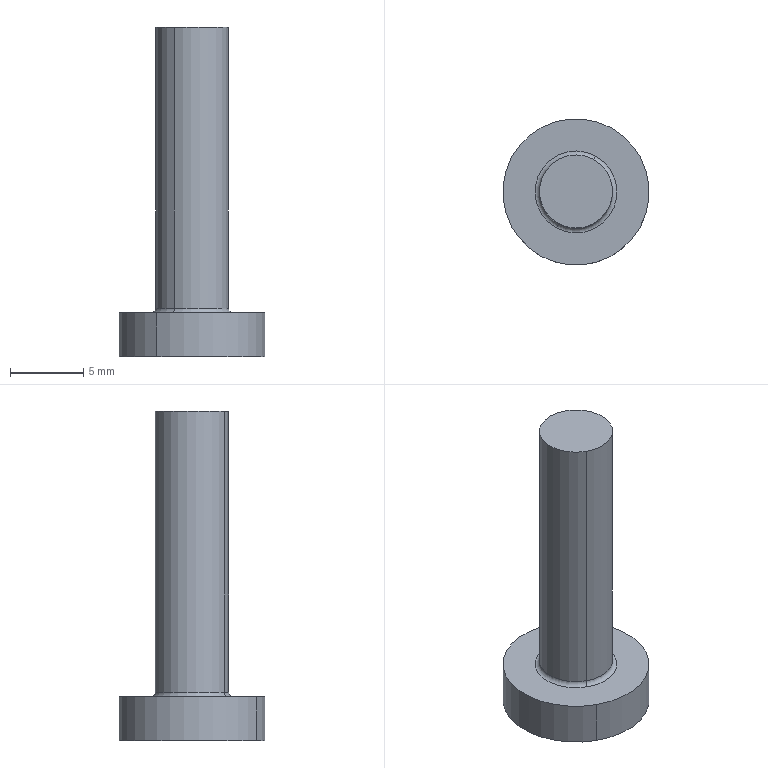Part | CATIA | 1 solid | 9 faces | box 10 x 10 x 22.5 mm | volume 618.813 mm3 | cylinder 4 | plane 3 | torus 2 | commonest cylinder face diameters 5 x2 10 x2
STEP:
#1=CARTESIAN_POINT('',(2.397,4.388,-3.));
#2=VERTEX_POINT('',#1);
#3=CARTESIAN_POINT('',(-2.397,-4.388,-3.));
#4=VERTEX_POINT('',#3);
#5=CARTESIAN_POINT('',(0.,0.,-3.));
#6=DIRECTION('',(0.,0.,-1.));
#7=AXIS2_PLACEMENT_3D('',#5,#6,$);
#8=CIRCLE('',#7,5.);
#9=EDGE_CURVE('',#2,#4,#8,.T.);
#10=ORIENTED_EDGE('',*,*,#9,.F.);
#11=CARTESIAN_POINT('',(2.397,4.388,0.));
#12=VERTEX_POINT('',#11);
#13=CARTESIAN_POINT('',(2.397,4.388,-1.5));
#14=DIRECTION('',(0.,0.,-1.));
#15=VECTOR('',#14,1.);
#16=LINE('',#13,#15);
#17=EDGE_CURVE('',#2,#12,#16,.F.);
#18=ORIENTED_EDGE('',*,*,#17,.T.);
#19=CARTESIAN_POINT('',(-2.397,-4.388,0.));
#20=VERTEX_POINT('',#19);
#21=CARTESIAN_POINT('',(0.,0.,0.));
#22=DIRECTION('',(0.,0.,-1.));
#23=AXIS2_PLACEMENT_3D('',#21,#22,$);
#24=CIRCLE('',#23,5.);
#25=EDGE_CURVE('',#12,#20,#24,.T.);
#26=ORIENTED_EDGE('',*,*,#25,.T.);
#27=CARTESIAN_POINT('',(-2.397,-4.388,-1.5));
#28=DIRECTION('',(0.,0.,-1.));
#29=VECTOR('',#28,1.);
#30=LINE('',#27,#29);
#31=EDGE_CURVE('',#4,#20,#30,.F.);
#32=ORIENTED_EDGE('',*,*,#31,.F.);
#33=EDGE_LOOP('',(#10,#18,#26,#32));
#34=FACE_OUTER_BOUND('',#33,.T.);
#35=CARTESIAN_POINT('',(0.,0.,8.25));
#36=DIRECTION('',(0.,0.,-1.));
#37=DIRECTION('',(0.4794,0.8776,0.));
#38=AXIS2_PLACEMENT_3D('',#35,#36,#37);
#39=CYLINDRICAL_SURFACE('',#38,5.);
#40=ADVANCED_FACE('',(#34),#39,.T.);
#41=CARTESIAN_POINT('',(0.,0.,-3.));
#42=DIRECTION('',(0.,0.,-1.));
#43=AXIS2_PLACEMENT_3D('',#41,#42,$);
#44=CIRCLE('',#43,5.);
#45=EDGE_CURVE('',#4,#2,#44,.T.);
#46=ORIENTED_EDGE('',*,*,#45,.F.);
#47=ORIENTED_EDGE('',*,*,#31,.T.);
#48=CARTESIAN_POINT('',(0.,0.,0.));
#49=DIRECTION('',(0.,0.,-1.));
#50=AXIS2_PLACEMENT_3D('',#48,#49,$);
#51=CIRCLE('',#50,5.);
#52=EDGE_CURVE('',#20,#12,#51,.T.);
#53=ORIENTED_EDGE('',*,*,#52,.T.);
#54=ORIENTED_EDGE('',*,*,#17,.F.);
#55=EDGE_LOOP('',(#46,#47,#53,#54));
#56=FACE_OUTER_BOUND('',#55,.T.);
#57=ADVANCED_FACE('',(#56),#39,.T.);
#58=CARTESIAN_POINT('',(1.342,2.457,0.));
#59=VERTEX_POINT('',#58);
#60=CARTESIAN_POINT('',(-1.342,-2.457,0.));
#61=VERTEX_POINT('',#60);
#62=CARTESIAN_POINT('',(0.,0.,0.));
#63=DIRECTION('',(0.,0.,-1.));
#64=AXIS2_PLACEMENT_3D('',#62,#63,$);
#65=CIRCLE('',#64,2.8);
#66=EDGE_CURVE('',#59,#61,#65,.T.);
#67=ORIENTED_EDGE('',*,*,#66,.F.);
#68=CARTESIAN_POINT('',(1.199,2.194,0.3));
#69=VERTEX_POINT('',#68);
#70=CARTESIAN_POINT('',(1.342,2.457,0.3));
#71=DIRECTION('',(-0.8776,0.4794,0.));
#72=AXIS2_PLACEMENT_3D('',#70,#71,$);
#73=CIRCLE('',#72,0.3);
#74=EDGE_CURVE('',#59,#69,#73,.T.);
#75=ORIENTED_EDGE('',*,*,#74,.T.);
#76=CARTESIAN_POINT('',(-1.199,-2.194,0.3));
#77=VERTEX_POINT('',#76);
#78=CARTESIAN_POINT('',(0.,0.,0.3));
#79=DIRECTION('',(0.,0.,-1.));
#80=AXIS2_PLACEMENT_3D('',#78,#79,$);
#81=CIRCLE('',#80,2.5);
#82=EDGE_CURVE('',#69,#77,#81,.T.);
#83=ORIENTED_EDGE('',*,*,#82,.T.);
#84=CARTESIAN_POINT('',(-1.342,-2.457,0.3));
#85=DIRECTION('',(0.8776,-0.4794,0.));
#86=AXIS2_PLACEMENT_3D('',#84,#85,$);
#87=CIRCLE('',#86,0.3);
#88=EDGE_CURVE('',#61,#77,#87,.T.);
#89=ORIENTED_EDGE('',*,*,#88,.F.);
#90=EDGE_LOOP('',(#67,#75,#83,#89));
#91=FACE_OUTER_BOUND('',#90,.T.);
#92=CARTESIAN_POINT('',(0.,0.,0.3));
#93=DIRECTION('',(0.,0.,-1.));
#94=DIRECTION('',(0.4794,0.8776,0.));
#95=AXIS2_PLACEMENT_3D('',#92,#93,#94);
#96=TOROIDAL_SURFACE('',#95,2.8,0.3);
#97=ADVANCED_FACE('',(#91),#96,.F.);
#98=CARTESIAN_POINT('',(0.,0.,0.));
#99=DIRECTION('',(0.,0.,-1.));
#100=AXIS2_PLACEMENT_3D('',#98,#99,$);
#101=CIRCLE('',#100,2.8);
#102=EDGE_CURVE('',#61,#59,#101,.T.);
#103=ORIENTED_EDGE('',*,*,#102,.F.);
#104=ORIENTED_EDGE('',*,*,#88,.T.);
#105=CARTESIAN_POINT('',(0.,0.,0.3));
#106=DIRECTION('',(0.,0.,-1.));
#107=AXIS2_PLACEMENT_3D('',#105,#106,$);
#108=CIRCLE('',#107,2.5);
#109=EDGE_CURVE('',#77,#69,#108,.T.);
#110=ORIENTED_EDGE('',*,*,#109,.T.);
#111=ORIENTED_EDGE('',*,*,#74,.F.);
#112=EDGE_LOOP('',(#103,#104,#110,#111));
#113=FACE_OUTER_BOUND('',#112,.T.);
#114=ADVANCED_FACE('',(#113),#96,.F.);
#115=ORIENTED_EDGE('',*,*,#82,.F.);
#116=CARTESIAN_POINT('',(1.199,2.194,19.5));
#117=VERTEX_POINT('',#116);
#118=CARTESIAN_POINT('',(1.199,2.194,9.9));
#119=DIRECTION('',(0.,0.,-1.));
#120=VECTOR('',#119,1.);
#121=LINE('',#118,#120);
#122=EDGE_CURVE('',#69,#117,#121,.F.);
#123=ORIENTED_EDGE('',*,*,#122,.T.);
#124=CARTESIAN_POINT('',(-1.199,-2.194,19.5));
#125=VERTEX_POINT('',#124);
#126=CARTESIAN_POINT('',(0.,0.,19.5));
#127=DIRECTION('',(0.,0.,-1.));
#128=AXIS2_PLACEMENT_3D('',#126,#127,$);
#129=CIRCLE('',#128,2.5);
#130=EDGE_CURVE('',#117,#125,#129,.T.);
#131=ORIENTED_EDGE('',*,*,#130,.T.);
#132=CARTESIAN_POINT('',(-1.199,-2.194,9.9));
#133=DIRECTION('',(0.,0.,-1.));
#134=VECTOR('',#133,1.);
#135=LINE('',#132,#134);
#136=EDGE_CURVE('',#77,#125,#135,.F.);
#137=ORIENTED_EDGE('',*,*,#136,.F.);
#138=EDGE_LOOP('',(#115,#123,#131,#137));
#139=FACE_OUTER_BOUND('',#138,.T.);
#140=CARTESIAN_POINT('',(0.,0.,8.25));
#141=DIRECTION('',(0.,0.,-1.));
#142=DIRECTION('',(0.4794,0.8776,0.));
#143=AXIS2_PLACEMENT_3D('',#140,#141,#142);
#144=CYLINDRICAL_SURFACE('',#143,2.5);
#145=ADVANCED_FACE('',(#139),#144,.T.);
#146=ORIENTED_EDGE('',*,*,#109,.F.);
#147=ORIENTED_EDGE('',*,*,#136,.T.);
#148=CARTESIAN_POINT('',(0.,0.,19.5));
#149=DIRECTION('',(0.,0.,-1.));
#150=AXIS2_PLACEMENT_3D('',#148,#149,$);
#151=CIRCLE('',#150,2.5);
#152=EDGE_CURVE('',#125,#117,#151,.T.);
#153=ORIENTED_EDGE('',*,*,#152,.T.);
#154=ORIENTED_EDGE('',*,*,#122,.F.);
#155=EDGE_LOOP('',(#146,#147,#153,#154));
#156=FACE_OUTER_BOUND('',#155,.T.);
#157=ADVANCED_FACE('',(#156),#144,.T.);
#158=ORIENTED_EDGE('',*,*,#9,.T.);
#159=ORIENTED_EDGE('',*,*,#45,.T.);
#160=EDGE_LOOP('',(#158,#159));
#161=FACE_OUTER_BOUND('',#160,.T.);
#162=CARTESIAN_POINT('',(0.,0.,-3.));
#163=DIRECTION('',(0.,0.,-1.));
#164=DIRECTION('',(1.,0.,0.));
#165=AXIS2_PLACEMENT_3D('',#162,#163,#164);
#166=PLANE('',#165);
#167=ADVANCED_FACE('',(#161),#166,.T.);
#168=ORIENTED_EDGE('',*,*,#25,.F.);
#169=ORIENTED_EDGE('',*,*,#52,.F.);
#170=EDGE_LOOP('',(#168,#169));
#171=FACE_OUTER_BOUND('',#170,.T.);
#172=ORIENTED_EDGE('',*,*,#102,.T.);
#173=ORIENTED_EDGE('',*,*,#66,.T.);
#174=EDGE_LOOP('',(#172,#173));
#175=FACE_BOUND('',#174,.T.);
#176=CARTESIAN_POINT('',(0.,5.,0.));
#177=DIRECTION('',(0.,0.,-1.));
#178=DIRECTION('',(1.,0.,0.));
#179=AXIS2_PLACEMENT_3D('',#176,#177,#178);
#180=PLANE('',#179);
#181=ADVANCED_FACE('',(#171,#175),#180,.F.);
#182=ORIENTED_EDGE('',*,*,#130,.F.);
#183=ORIENTED_EDGE('',*,*,#152,.F.);
#184=EDGE_LOOP('',(#182,#183));
#185=FACE_OUTER_BOUND('',#184,.T.);
#186=CARTESIAN_POINT('',(0.,2.5,19.5));
#187=DIRECTION('',(0.,0.,-1.));
#188=DIRECTION('',(1.,0.,0.));
#189=AXIS2_PLACEMENT_3D('',#186,#187,#188);
#190=PLANE('',#189);
#191=ADVANCED_FACE('',(#185),#190,.F.);
#192=CLOSED_SHELL('',(#40,#57,#97,#114,#145,#157,#167,#181,#191));
#193=MANIFOLD_SOLID_BREP('',#192);
#194=(LENGTH_UNIT()NAMED_UNIT(*)SI_UNIT(.MILLI.,.METRE.));
#195=UNCERTAINTY_MEASURE_WITH_UNIT(LENGTH_MEASURE(0.005),#194,'','');
#196=(NAMED_UNIT(*)PLANE_ANGLE_UNIT()SI_UNIT($,.RADIAN.));
#197=(NAMED_UNIT(*)SI_UNIT($,.STERADIAN.)SOLID_ANGLE_UNIT());
#198=(GEOMETRIC_REPRESENTATION_CONTEXT(3)GLOBAL_UNCERTAINTY_ASSIGNED_CONTEXT((#195))GLOBAL_UNIT_ASSIGNED_CONTEXT((#194,#196,#197))REPRESENTATION_CONTEXT('',''));
#199=ADVANCED_BREP_SHAPE_REPRESENTATION('',(#193),#198);